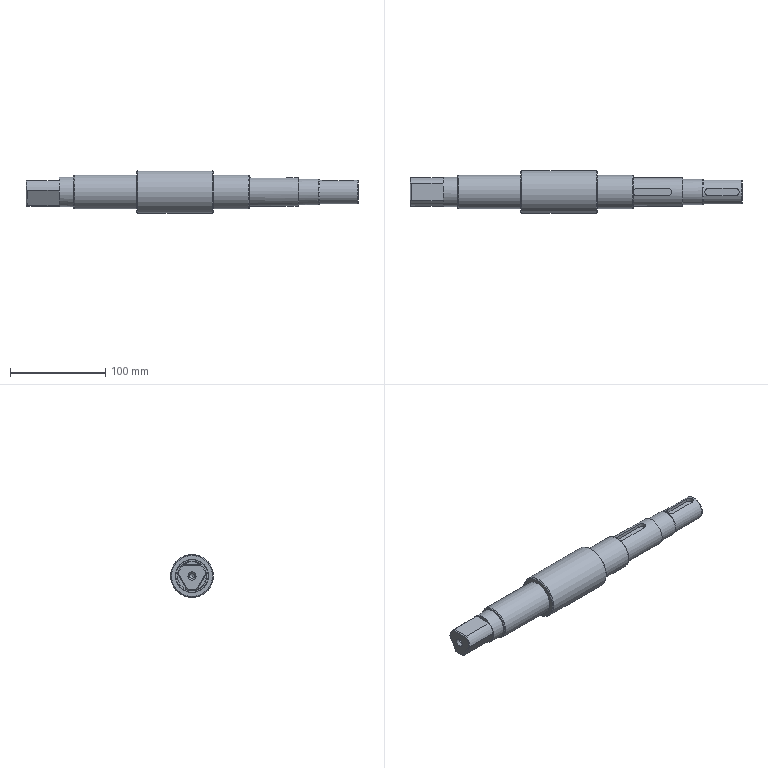NC program | NX | posted with a generic post | part box 348.4 x 45 x 45 mm
Lines 26 to 881 of 8230:
(ZLEVEL_PROFILE , TOOL : D12)
N44 T12 M6
N46 G54
N48 G17 G0 G90 X1.494 Y-21.088 B0. C0. S3000 M3
N50 G43 Z30. H12
N52 Z3.
N54 G94 G1 X0.322 Y-21.168 Z2.969 F1000.
N56 X-0.867 Y-21.132 Z2.938
N58 X-2.032 Y-21.052 Z2.908
N60 X-3.191 Y-20.908 Z2.877
N62 X-3.454 Y-20.866 Z2.87
N64 X-5.417 Y-20.445 Z2.817
N66 X-6.627 Y-20.109 Z2.785
N68 X-6.926 Y-20.009 Z2.776
N70 X-8.672 Y-19.316 Z2.727
N72 X-9.737 Y-18.63 Z2.694
N74 X-10.648 Y-17.751 Z2.661
N76 X-11.005 Y-17.24 Z2.644
N78 X-20.329 Y-1.089 Z2.156
N80 X-20.615 Y-0.558 Z2.14
N82 X-20.993 Y0.754 Z2.105
N84 X-21.068 Y2.117 Z2.069
N86 X-20.974 Y2.712 Z2.053
N88 X-20.913 Y3.155 Z2.041
N90 X-20.759 Y4.101 Z2.016
N92 X-20.487 Y5.346 Z1.983
N94 X-19.903 Y7.245 Z1.931
N96 X-19.428 Y8.428 Z1.897
N98 X-18.84 Y9.668 Z1.861
N100 X-18.585 Y10.139 Z1.847
N102 X-17.871 Y11.312 Z1.811
N104 X-17.235 Y12.297 Z1.781
N106 X-16.077 Y13.775 Z1.732
N108 X-14.802 Y15.153 Z1.682
N110 X-13.929 Y15.937 Z1.652
N112 X-12.824 Y16.819 Z1.615
N114 X-12.649 Y16.951 Z1.609
N116 X-12.159 Y17.312 Z1.593
N118 X-10.915 Y17.876 Z1.557
N120 X-9.578 Y18.153 Z1.522
N122 X-8.97 Y18.15 Z1.506
N124 X9.215 Z1.029
N126 X9.824 Y18.127 Z1.013
N128 X11.056 Y17.828 Z0.98
N130 X12.202 Y17.286 Z0.947
N132 X12.69 Y16.92 Z0.931
N134 X13.605 Y16.224 Z0.901
N136 X15.197 Y14.736 Z0.844
N138 X16.634 Y13.098 Z0.787
N140 X17.902 Y11.327 Z0.73
N142 X18.473 Y10.329 Z0.7
N144 X19.156 Y9.011 Z0.661
N146 X19.696 Y7.705 Z0.624
N148 X19.848 Y7.306 Z0.613
N150 X20.415 Y5.527 Z0.564
N152 X20.715 Y4.405 Z0.533
N154 X20.838 Y3.786 Z0.517
N156 X21.068 Y2.023 Z0.47
N158 X20.986 Y0.776 Z0.438
N160 X20.663 Y-0.43 Z0.405
N162 X20.39 Y-0.984 Z0.389
N164 X11.114 Y-17.05 Z-0.097
N166 X10.802 Y-17.561 Z-0.113
N168 X9.86 Y-18.549 Z-0.149
N170 X8.718 Y-19.298 Z-0.184
N172 X8.159 Y-19.512 Z-0.2
N174 X7.072 Y-19.96 F2200.
N176 G2 X3.724 Y-20.82 R30.718
N178 X-0.867 Y-21.132 R23.572
N180 X-3.191 Y-20.908 R42.566
N182 G1 X-3.454 Y-20.866
N184 X-5.417 Y-20.445
N186 G2 X-8.093 Y-19.546 R26.263
N188 X-11.005 Y-17.24 R6.45
N190 G1 X-20.329 Y-1.089
N192 G2 X-20.974 Y2.712 R6.027
N194 G1 X-20.913 Y3.155
N196 X-20.759 Y4.101
N198 G2 X-19.428 Y8.428 R27.054
N200 X-17.871 Y11.312 R31.394
N202 X-13.929 Y15.937 R22.915
N204 G1 X-12.824 Y16.819
N206 X-12.649 Y16.951
N208 G2 X-8.97 Y18.15 R6.146
N210 G1 X9.215
N212 G2 X12.69 Y16.92 R6.187
N214 X18.473 Y10.329 R22.033
N216 X19.696 Y7.705 R33.258
N218 G1 X19.848 Y7.306
N220 X20.415 Y5.527
N222 G2 X20.988 Y2.635 R22.446
N224 X20.39 Y-0.984 R6.331
N226 G1 X11.114 Y-17.05
N228 G2 X8.159 Y-19.512 R5.953
N230 G1 X7.78 Y-19.667 Z-0.207
N232 X7.395 Y-19.808 Z-0.214
N234 X7.009 Y-19.939 Z-0.221
N236 X6.625 Y-20.074 Z-0.229
N238 X6.238 Y-20.209 Z-0.236
N240 X5.846 Y-20.326 Z-0.243
N242 X5.451 Y-20.434 Z-0.25
N244 X5.051 Y-20.52 Z-0.257
N246 X4.651 Y-20.609 Z-0.264
N248 X4.252 Y-20.698 Z-0.271
N250 X3.853 Y-20.789 Z-0.279
N252 X3.451 Y-20.867 Z-0.286
N254 X3.046 Y-20.922 Z-0.293
N256 X2.639 Y-20.965 Z-0.3
N258 X2.232 Y-21.01 Z-0.307
N260 X1.826 Y-21.055 Z-0.314
N262 X1.418 Y-21.1 Z-0.321
N264 X1.01 Y-21.125 Z-0.329
N266 X0.601 Y-21.13 Z-0.336
N268 X0.191 Y-21.128 Z-0.343
N270 X-0.218 Z-0.35
N272 X-0.627 Y-21.13 Z-0.357
N274 X-1.036 Y-21.124 Z-0.364
N276 X-1.444 Y-21.098 Z-0.371
N278 X-1.851 Y-21.052 Z-0.379
N280 X-2.258 Y-21.007 Z-0.386
N282 X-2.665 Y-20.962 Z-0.393
N284 X-3.072 Y-20.923 Z-0.4
N286 X-3.191 Y-20.908
N288 X-3.454 Y-20.866
N290 X-5.417 Y-20.445
N292 G2 X-8.095 Y-19.545 R26.183
N294 X-11.004 Y-17.24 R6.449
N296 G1 X-20.329 Y-1.089
N298 G2 X-20.974 Y2.712 R6.027
N300 G1 X-20.913 Y3.155
N302 X-20.759 Y4.101
N304 G2 X-19.428 Y8.429 R27.032
N306 X-17.871 Y11.312 R31.353
N308 X-13.926 Y15.939 R22.888
N310 G1 X-12.824 Y16.819
N312 X-12.649 Y16.951
N314 G2 X-8.97 Y18.15 R6.146
N316 G1 X9.215
N318 G2 X12.69 Y16.92 R6.187
N320 X18.475 Y10.326 R22.025
N322 X19.696 Y7.705 R33.111
N324 G1 X19.848 Y7.306
N326 X20.415 Y5.527
N328 G2 X20.988 Y2.634 R22.427
N330 X20.39 Y-0.983 R6.332
N332 G1 X11.114 Y-17.05
N334 G2 X8.159 Y-19.512 R5.953
N336 G1 X7.78 Y-19.667 Z-0.407
N338 X7.395 Y-19.808 Z-0.414
N340 X7.009 Y-19.939 Z-0.421
N342 X6.625 Y-20.074 Z-0.429
N344 X6.238 Y-20.209 Z-0.436
N346 X5.846 Y-20.326 Z-0.443
N348 X5.451 Y-20.434 Z-0.45
N350 X5.051 Y-20.52 Z-0.457
N352 X4.651 Y-20.609 Z-0.464
N354 X4.252 Y-20.698 Z-0.471
N356 X3.853 Y-20.79 Z-0.479
N358 X3.451 Y-20.867 Z-0.486
N360 X3.046 Y-20.922 Z-0.493
N362 X2.639 Y-20.965 Z-0.5
N364 X2.232 Y-21.01 Z-0.507
N366 X1.826 Y-21.055 Z-0.514
N368 X1.419 Y-21.101 Z-0.521
N370 X1.01 Y-21.125 Z-0.529
N372 X0.601 Y-21.13 Z-0.536
N374 X0.191 Y-21.128 Z-0.543
N376 X-0.218 Z-0.55
N378 X-0.627 Y-21.13 Z-0.557
N380 X-1.036 Y-21.124 Z-0.564
N382 X-1.444 Y-21.098 Z-0.571
N384 X-1.851 Y-21.052 Z-0.579
N386 X-2.258 Y-21.007 Z-0.586
N388 X-2.665 Y-20.962 Z-0.593
N390 X-3.072 Y-20.923 Z-0.6
N392 X-3.191 Y-20.908
N394 X-3.454 Y-20.866
N396 X-5.417 Y-20.445
N398 G2 X-8.097 Y-19.544 R26.105
N400 X-11.004 Y-17.24 R6.448
N402 G1 X-20.329 Y-1.089
N404 G2 X-20.974 Y2.712 R6.027
N406 G1 X-20.913 Y3.155
N408 X-20.759 Y4.101
N410 G2 X-19.427 Y8.43 R27.01
N412 X-17.871 Y11.312 R31.313
N414 X-13.923 Y15.942 R22.861
N416 G1 X-12.824 Y16.819
N418 X-12.649 Y16.951
N420 G2 X-8.97 Y18.15 R6.146
N422 G1 X9.215
N424 G2 X12.69 Y16.92 R6.186
N426 X18.476 Y10.324 R22.016
N428 X19.696 Y7.705 R32.965
N430 G1 X19.848 Y7.306
N432 X20.415 Y5.527
N434 G2 X20.988 Y2.633 R22.408
N436 X20.39 Y-0.983 R6.332
N438 G1 X11.114 Y-17.05
N440 G2 X8.159 Y-19.512 R5.953
N442 G1 X7.78 Y-19.667 Z-0.607
N444 X7.396 Y-19.808 Z-0.614
N446 X7.009 Y-19.939 Z-0.621
N448 X6.625 Y-20.075 Z-0.629
N450 X6.237 Y-20.208 Z-0.636
N452 X5.846 Y-20.326 Z-0.643
N454 X5.451 Y-20.434 Z-0.65
N456 X5.051 Y-20.521 Z-0.657
N458 X4.651 Y-20.61 Z-0.664
N460 X4.252 Y-20.698 Z-0.671
N462 X3.853 Y-20.789 Z-0.679
N464 X3.451 Y-20.867 Z-0.686
N466 X3.046 Y-20.923 Z-0.693
N468 X2.639 Y-20.965 Z-0.7
N470 X2.232 Y-21.01 Z-0.707
N472 X1.826 Y-21.054 Z-0.714
N474 X1.419 Y-21.101 Z-0.721
N476 X1.01 Y-21.125 Z-0.729
N478 X0.601 Y-21.13 Z-0.736
N480 X0.191 Y-21.128 Z-0.743
N482 X-0.218 Z-0.75
N484 X-0.627 Y-21.13 Z-0.757
N486 X-1.036 Y-21.124 Z-0.764
N488 X-1.444 Y-21.098 Z-0.771
N490 X-1.851 Y-21.052 Z-0.779
N492 X-2.258 Y-21.007 Z-0.786
N494 X-2.665 Y-20.962 Z-0.793
N496 X-3.072 Y-20.923 Z-0.8
N498 X-3.191 Y-20.908
N500 X-3.454 Y-20.866
N502 X-5.417 Y-20.445
N504 G2 X-8.099 Y-19.543 R26.026
N506 X-11.004 Y-17.24 R6.447
N508 G1 X-20.329 Y-1.089
N510 G2 X-20.974 Y2.712 R6.027
N512 G1 X-20.913 Y3.155
N514 X-20.759 Y4.101
N516 G2 X-19.427 Y8.431 R26.988
N518 X-17.871 Y11.312 R31.273
N520 X-13.919 Y15.945 R22.834
N522 G1 X-12.824 Y16.819
N524 X-12.649 Y16.951
N526 G2 X-8.97 Y18.15 R6.146
N528 G1 X9.215
N530 G2 X12.69 Y16.92 R6.186
N532 X18.477 Y10.321 R22.007
N534 X19.696 Y7.705 R32.82
N536 G1 X19.848 Y7.306
N538 X20.415 Y5.527
N540 G2 X20.988 Y2.633 R22.389
N542 X20.391 Y-0.982 R6.332
N544 G1 X11.114 Y-17.05
N546 G2 X8.159 Y-19.512 R5.953
N548 G1 X7.78 Y-19.667 Z-0.807
N550 X7.395 Y-19.808 Z-0.814
N552 X7.009 Y-19.94 Z-0.821
N554 X6.625 Y-20.074 Z-0.829
N556 X6.237 Y-20.208 Z-0.836
N558 X5.846 Y-20.326 Z-0.843
N560 X5.451 Y-20.433 Z-0.85
N562 X5.051 Y-20.521 Z-0.857
N564 X4.651 Y-20.61 Z-0.864
N566 X4.252 Y-20.698 Z-0.871
N568 X3.853 Y-20.789 Z-0.879
N570 X3.451 Y-20.867 Z-0.886
N572 X3.046 Y-20.923 Z-0.893
N574 X2.639 Y-20.965 Z-0.9
N576 X2.232 Y-21.009 Z-0.907
N578 X1.826 Y-21.055 Z-0.914
N580 X1.419 Y-21.101 Z-0.921
N582 X1.01 Y-21.125 Z-0.929
N584 X0.601 Y-21.13 Z-0.936
N586 X0.192 Y-21.138 Z-0.943
N588 X-0.218 Y-21.14 Z-0.95
N590 X-0.627 Y-21.134 Z-0.957
N592 X-1.036 Y-21.124 Z-0.964
N594 X-1.444 Y-21.099 Z-0.971
N596 X-1.853 Y-21.067 Z-0.979
N598 X-2.26 Y-21.027 Z-0.986
N600 X-2.666 Y-20.98 Z-0.993
N602 X-3.072 Y-20.926 Z-1.
N604 G2 X-8.273 Y-19.465 R21.135
N606 X-11.134 Y-17.015 R6.16
N608 G1 X-20.329 Y-1.089
N610 G2 X-20.974 Y2.712 R6.027
N612 G1 X-20.909 Y3.178
N614 X-20.881 Y3.365
N616 G2 X-12.649 Y16.951 R21.153
N618 X-8.97 Y18.15 R6.146
N620 G1 X9.215
N622 G2 X12.69 Y16.92 R6.186
N624 X20.995 Y2.56 R21.15
N626 X20.839 Y0.226 R6.123
N628 X20.203 Y-1.307 R6.281
N630 G1 X11.114 Y-17.05
N632 G2 X8.159 Y-19.512 R5.953
N634 G1 X7.78 Y-19.667 Z-1.007
N636 X7.398 Y-19.814 Z-1.014
N638 X7.013 Y-19.953 Z-1.021
N640 X6.626 Y-20.085 Z-1.029
N642 X6.236 Y-20.21 Z-1.036
N644 X5.844 Y-20.327 Z-1.043
N646 X5.449 Y-20.436 Z-1.05
N648 X5.053 Y-20.538 Z-1.057
N650 X4.655 Y-20.631 Z-1.064
N652 X4.255 Y-20.718 Z-1.071
N654 X3.853 Y-20.796 Z-1.079
N656 X3.45 Y-20.867 Z-1.086
N658 X3.046 Y-20.93 Z-1.093
N660 X2.64 Y-20.985 Z-1.1
N662 X2.234 Y-21.032 Z-1.107
N664 X1.826 Y-21.071 Z-1.114
N666 X1.418 Y-21.102 Z-1.121
N668 X1.01 Y-21.126 Z-1.129
N670 X0.601 Y-21.141 Z-1.136
N672 X0.192 Y-21.149 Z-1.143
N674 X-0.218 Z-1.15
N676 X-0.627 Y-21.141 Z-1.157
N678 X-1.036 Y-21.125 Z-1.164
N680 X-1.444 Y-21.101 Z-1.171
N682 X-1.852 Y-21.069 Z-1.179
N684 X-2.259 Y-21.029 Z-1.186
N686 X-2.666 Y-20.981 Z-1.193
N688 X-3.071 Y-20.926 Z-1.2
N690 G2 X-8.273 Y-19.465 R21.15
N692 X-11.135 Y-17.013 R6.159
N694 G1 X-20.329 Y-1.089
N696 G2 X-20.974 Y2.712 R6.027
N698 G1 X-20.958 Y2.84
N700 G2 X-12.824 Y16.819 R21.15
N702 X-9.005 Y18.15 R6.32
N704 G1 X9.215
N706 G2 X12.671 Y16.934 R6.186
N708 X20.995 Y2.56 R21.15
N710 X20.839 Y0.226 R5.624
N712 X20.203 Y-1.307 R6.717
N714 G1 X11.114 Y-17.05
N716 G2 X8.159 Y-19.512 R5.953
N718 G1 X7.78 Y-19.667 Z-1.207
N720 X7.398 Y-19.814 Z-1.214
N722 X7.013 Y-19.953 Z-1.221
N724 X6.626 Y-20.085 Z-1.229
N726 X6.236 Y-20.21 Z-1.236
N728 X5.844 Y-20.327 Z-1.243
N730 X5.45 Y-20.436 Z-1.25
N732 X5.053 Y-20.537 Z-1.257
N734 X4.655 Y-20.631 Z-1.264
N736 X4.255 Y-20.718 Z-1.271
N738 X3.853 Y-20.796 Z-1.279
N740 X3.45 Y-20.867 Z-1.286
N742 X3.046 Y-20.93 Z-1.293
N744 X2.64 Y-20.985 Z-1.3
N746 X2.234 Y-21.032 Z-1.307
N748 X1.827 Y-21.071 Z-1.314
N750 X1.419 Y-21.102 Z-1.321
N752 X1.01 Y-21.126 Z-1.329
N754 X0.601 Y-21.141 Z-1.336
N756 X0.192 Y-21.149 Z-1.343
N758 X-0.217 Z-1.35
N760 X-0.626 Y-21.141 Z-1.357
N762 X-1.035 Y-21.125 Z-1.364
N764 X-1.444 Y-21.101 Z-1.371
N766 X-1.852 Y-21.069 Z-1.379
N768 X-2.259 Y-21.029 Z-1.386
N770 X-2.665 Y-20.981 Z-1.393
N772 X-3.071 Y-20.926 Z-1.4
N774 G2 X-8.273 Y-19.465 R21.15
N776 X-11.136 Y-17.012 R6.159
N778 G1 X-20.329 Y-1.089
N780 G2 X-20.985 Y2.636 R5.935
N782 X-12.776 Y16.855 R21.15
N784 X-9.005 Y18.15 R6.257
N786 G1 X9.215
N788 G2 X12.673 Y16.933 R6.185
N790 X20.995 Y2.56 R21.15
N792 X20.839 Y0.226 R5.624
N794 X20.203 Y-1.307 R6.717
N796 G1 X11.114 Y-17.05
N798 G2 X8.159 Y-19.513 R5.955
N800 G1 X7.78 Y-19.667 Z-1.407
N802 X7.398 Y-19.814 Z-1.414
N804 X7.013 Y-19.953 Z-1.421
N806 X6.626 Y-20.085 Z-1.429
N808 X6.236 Y-20.21 Z-1.436
N810 X5.844 Y-20.327 Z-1.443
N812 X5.45 Y-20.436 Z-1.45
N814 X5.053 Y-20.537 Z-1.457
N816 X4.655 Y-20.631 Z-1.464
N818 X4.255 Y-20.718 Z-1.471
N820 X3.853 Y-20.796 Z-1.479
N822 X3.45 Y-20.867 Z-1.486
N824 X3.046 Y-20.93 Z-1.493
N826 X2.64 Y-20.985 Z-1.5
N828 X2.234 Y-21.032 Z-1.507
N830 X1.827 Y-21.071 Z-1.514
N832 X1.419 Y-21.102 Z-1.521
N834 X1.01 Y-21.126 Z-1.529
N836 X0.601 Y-21.141 Z-1.536
N838 X0.192 Y-21.149 Z-1.543
N840 X-0.217 Z-1.55
N842 X-0.626 Y-21.141 Z-1.557
N844 X-1.035 Y-21.125 Z-1.564
N846 X-1.444 Y-21.101 Z-1.571
N848 X-1.852 Y-21.069 Z-1.579
N850 X-2.259 Y-21.029 Z-1.586
N852 X-2.665 Y-20.981 Z-1.593
N854 X-3.071 Y-20.926 Z-1.6
N856 G2 X-8.308 Y-19.45 R21.15
N858 X-11.218 Y-16.869 R6.15
N860 G1 X-20.22 Y-1.279
N862 G2 X-20.998 Y2.53 R6.15
N864 X-12.69 Y16.92 R21.15
N866 X-8.97 Y18.15 R6.15
N868 G1 X9.
N870 G2 X12.69 Y16.92 R6.15
N872 X20.998 Y2.53 R21.15
N874 X20.218 Y-1.281 R6.15
N876 G1 X11.218 Y-16.87
N878 G2 X8.308 Y-19.45 R6.15
N880 G1 X8.159 Y-19.513
N882 X7.78 Y-19.667 Z-1.607
N884 X7.398 Y-19.814 Z-1.614
N886 X7.013 Y-19.953 Z-1.621
N888 X6.626 Y-20.085 Z-1.629
N890 X6.236 Y-20.21 Z-1.636
N892 X5.844 Y-20.327 Z-1.643
N894 X5.45 Y-20.436 Z-1.65
N896 X5.053 Y-20.537 Z-1.657
N898 X4.655 Y-20.631 Z-1.664
N900 X4.255 Y-20.718 Z-1.671
N902 X3.853 Y-20.796 Z-1.679
N904 X3.45 Y-20.867 Z-1.686
N906 X3.046 Y-20.93 Z-1.693
N908 X2.64 Y-20.985 Z-1.7
N910 X2.234 Y-21.032 Z-1.707
N912 X1.827 Y-21.071 Z-1.714
N914 X1.419 Y-21.102 Z-1.721
N916 X1.01 Y-21.126 Z-1.729
N918 X0.601 Y-21.141 Z-1.736
N920 X0.192 Y-21.149 Z-1.743
N922 X-0.217 Z-1.75
N924 X-0.626 Y-21.141 Z-1.757
N926 X-1.035 Y-21.125 Z-1.764
N928 X-1.444 Y-21.101 Z-1.771
N930 X-1.852 Y-21.069 Z-1.779
N932 X-2.259 Y-21.029 Z-1.786
N934 X-2.665 Y-20.981 Z-1.793
N936 X-3.071 Y-20.926 Z-1.8
N938 G2 X-8.308 Y-19.45 R21.15
N940 X-11.218 Y-16.869 R6.15
N942 G1 X-20.22 Y-1.279
N944 G2 X-20.998 Y2.53 R6.15
N946 X-12.69 Y16.92 R21.15
N948 X-8.97 Y18.15 R6.15
N950 G1 X9.
N952 G2 X12.69 Y16.92 R6.15
N954 X20.998 Y2.53 R21.15
N956 X20.218 Y-1.281 R6.15
N958 G1 X11.218 Y-16.87
N960 G2 X8.308 Y-19.45 R6.15
N962 G1 X8.159 Y-19.513
N964 X7.78 Y-19.668 Z-1.807
N966 X7.398 Y-19.814 Z-1.814
N968 X7.013 Y-19.953 Z-1.821
N970 X6.626 Y-20.085 Z-1.829
N972 X6.236 Y-20.21 Z-1.836
N974 X5.844 Y-20.327 Z-1.843
N976 X5.45 Y-20.436 Z-1.85
N978 X5.053 Y-20.537 Z-1.857
N980 X4.655 Y-20.631 Z-1.864
N982 X4.255 Y-20.718 Z-1.871
N984 X3.853 Y-20.796 Z-1.879
N986 X3.45 Y-20.867 Z-1.886
N988 X3.046 Y-20.93 Z-1.893
N990 X2.64 Y-20.985 Z-1.9
N992 X2.234 Y-21.032 Z-1.907
N994 X1.827 Y-21.071 Z-1.914
N996 X1.419 Y-21.102 Z-1.921
N998 X1.01 Y-21.126 Z-1.929
N1000 X0.601 Y-21.141 Z-1.936
N1002 X0.192 Y-21.149 Z-1.943
N1004 X-0.217 Z-1.95
N1006 X-0.626 Y-21.141 Z-1.957
N1008 X-1.035 Y-21.125 Z-1.964
N1010 X-1.444 Y-21.101 Z-1.971
N1012 X-1.852 Y-21.069 Z-1.979
N1014 X-2.259 Y-21.029 Z-1.986
N1016 X-2.665 Y-20.981 Z-1.993
N1018 X-3.071 Y-20.926 Z-2.
N1020 G2 X-8.308 Y-19.45 R21.15
N1022 X-11.218 Y-16.869 R6.15
N1024 G1 X-20.22 Y-1.278
N1026 G2 X-20.998 Y2.53 R6.15
N1028 X-12.69 Y16.92 R21.15
N1030 X-8.97 Y18.15 R6.15
N1032 G1 X9.
N1034 G2 X12.69 Y16.92 R6.15
N1036 X20.998 Y2.53 R21.15
N1038 X20.218 Y-1.281 R6.15
N1040 G1 X11.218 Y-16.87
N1042 G2 X8.308 Y-19.45 R6.15
N1044 G1 X8.159 Y-19.513
N1046 X7.78 Y-19.668 Z-2.007
N1048 X7.398 Y-19.814 Z-2.014
N1050 X7.013 Y-19.953 Z-2.021
N1052 X6.626 Y-20.085 Z-2.029
N1054 X6.236 Y-20.21 Z-2.036
N1056 X5.844 Y-20.327 Z-2.043
N1058 X5.45 Y-20.436 Z-2.05
N1060 X5.053 Y-20.537 Z-2.057
N1062 X4.655 Y-20.631 Z-2.064
N1064 X4.255 Y-20.718 Z-2.071
N1066 X3.853 Y-20.796 Z-2.079
N1068 X3.45 Y-20.867 Z-2.086
N1070 X3.046 Y-20.93 Z-2.093
N1072 X2.64 Y-20.985 Z-2.1
N1074 X2.234 Y-21.032 Z-2.107
N1076 X1.827 Y-21.071 Z-2.114
N1078 X1.419 Y-21.102 Z-2.121
N1080 X1.01 Y-21.126 Z-2.129
N1082 X0.601 Y-21.141 Z-2.136
N1084 X0.192 Y-21.149 Z-2.143
N1086 X-0.217 Z-2.15
N1088 X-0.626 Y-21.141 Z-2.157
N1090 X-1.035 Y-21.125 Z-2.164
N1092 X-1.444 Y-21.101 Z-2.171
N1094 X-1.852 Y-21.069 Z-2.179
N1096 X-2.259 Y-21.029 Z-2.186
N1098 X-2.665 Y-20.981 Z-2.193
N1100 X-3.071 Y-20.926 Z-2.2
N1102 G2 X-8.308 Y-19.45 R21.15
N1104 X-11.218 Y-16.869 R6.15
N1106 G1 X-20.22 Y-1.278
N1108 G2 X-20.998 Y2.53 R6.15
N1110 X-12.69 Y16.92 R21.15
N1112 X-8.97 Y18.15 R6.15
N1114 G1 X9.
N1116 G2 X12.69 Y16.92 R6.15
N1118 X20.998 Y2.53 R21.15
N1120 X20.218 Y-1.281 R6.15
N1122 G1 X11.218 Y-16.87
N1124 G2 X8.308 Y-19.45 R6.15
N1126 G1 X8.159 Y-19.513
N1128 X7.78 Y-19.668 Z-2.207
N1130 X7.398 Y-19.814 Z-2.214
N1132 X7.013 Y-19.953 Z-2.221
N1134 X6.626 Y-20.085 Z-2.229
N1136 X6.236 Y-20.21 Z-2.236
N1138 X5.844 Y-20.327 Z-2.243
N1140 X5.45 Y-20.436 Z-2.25
N1142 X5.053 Y-20.537 Z-2.257
N1144 X4.655 Y-20.631 Z-2.264
N1146 X4.255 Y-20.718 Z-2.271
N1148 X3.853 Y-20.796 Z-2.279
N1150 X3.45 Y-20.867 Z-2.286
N1152 X3.046 Y-20.93 Z-2.293
N1154 X2.64 Y-20.985 Z-2.3
N1156 X2.234 Y-21.032 Z-2.307
N1158 X1.827 Y-21.071 Z-2.314
N1160 X1.419 Y-21.102 Z-2.321
N1162 X1.01 Y-21.126 Z-2.329
N1164 X0.601 Y-21.141 Z-2.336
N1166 X0.192 Y-21.149 Z-2.343
N1168 X-0.217 Z-2.35
N1170 X-0.626 Y-21.141 Z-2.357
N1172 X-1.035 Y-21.125 Z-2.364
N1174 X-1.444 Y-21.101 Z-2.371
N1176 X-1.852 Y-21.069 Z-2.379
N1178 X-2.259 Y-21.029 Z-2.386
N1180 X-2.665 Y-20.981 Z-2.393
N1182 X-3.071 Y-20.926 Z-2.4
N1184 G2 X-8.308 Y-19.45 R21.15
N1186 X-11.218 Y-16.869 R6.15
N1188 G1 X-20.22 Y-1.278
N1190 G2 X-20.998 Y2.53 R6.15
N1192 X-12.69 Y16.92 R21.15
N1194 X-8.97 Y18.15 R6.15
N1196 G1 X9.
N1198 G2 X12.69 Y16.92 R6.15
N1200 X20.998 Y2.53 R21.15
N1202 X20.218 Y-1.281 R6.15
N1204 G1 X11.218 Y-16.87
N1206 G2 X8.308 Y-19.45 R6.15
N1208 G1 X8.159 Y-19.513
N1210 X7.78 Y-19.668 Z-2.407
N1212 X7.398 Y-19.814 Z-2.414
N1214 X7.013 Y-19.953 Z-2.421
N1216 X6.626 Y-20.085 Z-2.429
N1218 X6.236 Y-20.21 Z-2.436
N1220 X5.844 Y-20.327 Z-2.443
N1222 X5.45 Y-20.436 Z-2.45
N1224 X5.053 Y-20.537 Z-2.457
N1226 X4.655 Y-20.631 Z-2.464
N1228 X4.255 Y-20.718 Z-2.471
N1230 X3.853 Y-20.796 Z-2.479
N1232 X3.45 Y-20.867 Z-2.486
N1234 X3.046 Y-20.93 Z-2.493
N1236 X2.64 Y-20.985 Z-2.5
N1238 X2.234 Y-21.032 Z-2.507
N1240 X1.827 Y-21.071 Z-2.514
N1242 X1.419 Y-21.102 Z-2.521
N1244 X1.01 Y-21.126 Z-2.529
N1246 X0.601 Y-21.141 Z-2.536
N1248 X0.192 Y-21.149 Z-2.543
N1250 X-0.217 Z-2.55
N1252 X-0.626 Y-21.141 Z-2.557
N1254 X-1.035 Y-21.125 Z-2.564
N1256 X-1.444 Y-21.101 Z-2.571
N1258 X-1.852 Y-21.069 Z-2.579
N1260 X-2.259 Y-21.029 Z-2.586
N1262 X-2.665 Y-20.981 Z-2.593
N1264 X-3.071 Y-20.926 Z-2.6
N1266 G2 X-8.308 Y-19.45 R21.15
N1268 X-11.218 Y-16.869 R6.15
N1270 G1 X-20.22 Y-1.278
N1272 G2 X-20.998 Y2.53 R6.15
N1274 X-12.69 Y16.92 R21.15
N1276 X-8.97 Y18.15 R6.15
N1278 G1 X9.
N1280 G2 X12.69 Y16.92 R6.15
N1282 X20.998 Y2.53 R21.15
N1284 X20.218 Y-1.281 R6.15
N1286 G1 X11.218 Y-16.871
N1288 G2 X8.308 Y-19.45 R6.15
N1290 G1 X8.159 Y-19.513
N1292 X7.78 Y-19.668 Z-2.607
N1294 X7.398 Y-19.814 Z-2.614
N1296 X7.013 Y-19.953 Z-2.621
N1298 X6.626 Y-20.085 Z-2.629
N1300 X6.236 Y-20.21 Z-2.636
N1302 X5.844 Y-20.327 Z-2.643
N1304 X5.45 Y-20.436 Z-2.65
N1306 X5.053 Y-20.537 Z-2.657
N1308 X4.655 Y-20.631 Z-2.664
N1310 X4.255 Y-20.718 Z-2.671
N1312 X3.853 Y-20.796 Z-2.679
N1314 X3.45 Y-20.867 Z-2.686
N1316 X3.046 Y-20.93 Z-2.693
N1318 X2.64 Y-20.985 Z-2.7
N1320 X2.234 Y-21.032 Z-2.707
N1322 X1.827 Y-21.071 Z-2.714
N1324 X1.419 Y-21.102 Z-2.721
N1326 X1.01 Y-21.126 Z-2.729
N1328 X0.601 Y-21.141 Z-2.736
N1330 X0.192 Y-21.149 Z-2.743
N1332 X-0.217 Z-2.75
N1334 X-0.626 Y-21.141 Z-2.757
N1336 X-1.035 Y-21.125 Z-2.764
N1338 X-1.444 Y-21.101 Z-2.771
N1340 X-1.852 Y-21.069 Z-2.779
N1342 X-2.259 Y-21.029 Z-2.786
N1344 X-2.665 Y-20.981 Z-2.793
N1346 X-3.071 Y-20.926 Z-2.8
N1348 G2 X-8.308 Y-19.45 R21.15
N1350 X-11.218 Y-16.869 R6.15
N1352 G1 X-20.22 Y-1.278
N1354 G2 X-20.998 Y2.53 R6.15
N1356 X-12.69 Y16.92 R21.15
N1358 X-8.97 Y18.15 R6.15
N1360 G1 X9.
N1362 G2 X12.69 Y16.92 R6.15
N1364 X20.998 Y2.53 R21.15
N1366 X20.218 Y-1.281 R6.15
N1368 G1 X11.218 Y-16.871
N1370 G2 X8.308 Y-19.45 R6.15
N1372 G1 X8.159 Y-19.513
N1374 X7.78 Y-19.668 Z-2.807
N1376 X7.398 Y-19.814 Z-2.814
N1378 X7.013 Y-19.953 Z-2.821
N1380 X6.626 Y-20.085 Z-2.829
N1382 X6.236 Y-20.21 Z-2.836
N1384 X5.844 Y-20.327 Z-2.843
N1386 X5.45 Y-20.436 Z-2.85
N1388 X5.053 Y-20.537 Z-2.857
N1390 X4.655 Y-20.631 Z-2.864
N1392 X4.255 Y-20.718 Z-2.871
N1394 X3.853 Y-20.796 Z-2.879
N1396 X3.45 Y-20.867 Z-2.886
N1398 X3.046 Y-20.93 Z-2.893
N1400 X2.64 Y-20.985 Z-2.9
N1402 X2.234 Y-21.032 Z-2.907
N1404 X1.827 Y-21.071 Z-2.914
N1406 X1.419 Y-21.102 Z-2.921
N1408 X1.01 Y-21.126 Z-2.929
N1410 X0.601 Y-21.141 Z-2.936
N1412 X0.192 Y-21.149 Z-2.943
N1414 X-0.217 Z-2.95
N1416 X-0.626 Y-21.141 Z-2.957
N1418 X-1.035 Y-21.125 Z-2.964
N1420 X-1.444 Y-21.101 Z-2.971
N1422 X-1.852 Y-21.069 Z-2.979
N1424 X-2.259 Y-21.029 Z-2.986
N1426 X-2.665 Y-20.981 Z-2.993
N1428 X-3.071 Y-20.926 Z-3.
N1430 G2 X-8.308 Y-19.45 R21.15
N1432 X-11.218 Y-16.869 R6.15
N1434 G1 X-20.22 Y-1.278
N1436 G2 X-20.998 Y2.53 R6.15
N1438 X-12.69 Y16.92 R21.15
N1440 X-8.97 Y18.15 R6.15
N1442 G1 X9.
N1444 G2 X12.69 Y16.92 R6.15
N1446 X20.998 Y2.53 R21.15
N1448 X20.218 Y-1.281 R6.15
N1450 G1 X11.217 Y-16.871
N1452 G2 X8.308 Y-19.45 R6.15
N1454 G1 X8.159 Y-19.513
N1456 X7.78 Y-19.668 Z-3.007
N1458 X7.398 Y-19.814 Z-3.014
N1460 X7.013 Y-19.953 Z-3.021
N1462 X6.626 Y-20.085 Z-3.029
N1464 X6.236 Y-20.21 Z-3.036
N1466 X5.844 Y-20.327 Z-3.043
N1468 X5.45 Y-20.436 Z-3.05
N1470 X5.053 Y-20.537 Z-3.057
N1472 X4.655 Y-20.631 Z-3.064
N1474 X4.255 Y-20.718 Z-3.071
N1476 X3.853 Y-20.796 Z-3.079
N1478 X3.45 Y-20.867 Z-3.086
N1480 X3.046 Y-20.93 Z-3.093
N1482 X2.64 Y-20.985 Z-3.1
N1484 X2.234 Y-21.032 Z-3.107
N1486 X1.827 Y-21.071 Z-3.114
N1488 X1.419 Y-21.102 Z-3.121
N1490 X1.01 Y-21.126 Z-3.129
N1492 X0.601 Y-21.141 Z-3.136
N1494 X0.192 Y-21.149 Z-3.143
N1496 X-0.217 Z-3.15
N1498 X-0.626 Y-21.141 Z-3.157
N1500 X-1.035 Y-21.125 Z-3.164
N1502 X-1.444 Y-21.101 Z-3.171
N1504 X-1.852 Y-21.069 Z-3.179
N1506 X-2.259 Y-21.029 Z-3.186
N1508 X-2.665 Y-20.981 Z-3.193
N1510 X-3.071 Y-20.926 Z-3.2
N1512 G2 X-8.308 Y-19.45 R21.15
N1514 X-11.218 Y-16.869 R6.15
N1516 G1 X-20.22 Y-1.278
N1518 G2 X-20.998 Y2.53 R6.15
N1520 X-12.69 Y16.92 R21.15
N1522 X-8.97 Y18.15 R6.15
N1524 G1 X9.
N1526 G2 X12.69 Y16.92 R6.15
N1528 X20.998 Y2.53 R21.15
N1530 X20.218 Y-1.281 R6.15
N1532 G1 X11.217 Y-16.871
N1534 G2 X8.308 Y-19.45 R6.15
N1536 G1 X8.159 Y-19.513
N1538 X7.78 Y-19.668 Z-3.207
N1540 X7.398 Y-19.814 Z-3.214
N1542 X7.013 Y-19.953 Z-3.221
N1544 X6.626 Y-20.085 Z-3.229
N1546 X6.236 Y-20.21 Z-3.236
N1548 X5.844 Y-20.327 Z-3.243
N1550 X5.45 Y-20.436 Z-3.25
N1552 X5.053 Y-20.537 Z-3.257
N1554 X4.655 Y-20.631 Z-3.264
N1556 X4.255 Y-20.718 Z-3.271
N1558 X3.853 Y-20.796 Z-3.279
N1560 X3.45 Y-20.867 Z-3.286
N1562 X3.046 Y-20.93 Z-3.293
N1564 X2.64 Y-20.985 Z-3.3
N1566 X2.234 Y-21.032 Z-3.307
N1568 X1.827 Y-21.071 Z-3.314
N1570 X1.419 Y-21.102 Z-3.321
N1572 X1.01 Y-21.126 Z-3.329
N1574 X0.601 Y-21.141 Z-3.336
N1576 X0.192 Y-21.149 Z-3.343
N1578 X-0.217 Z-3.35
N1580 X-0.626 Y-21.141 Z-3.357
N1582 X-1.035 Y-21.125 Z-3.364
N1584 X-1.444 Y-21.101 Z-3.371
N1586 X-1.852 Y-21.069 Z-3.379
N1588 X-2.259 Y-21.029 Z-3.386
N1590 X-2.665 Y-20.981 Z-3.393
N1592 X-3.071 Y-20.926 Z-3.4
N1594 G2 X-8.308 Y-19.45 R21.15
N1596 X-11.218 Y-16.869 R6.15
N1598 G1 X-20.22 Y-1.278
N1600 G2 X-20.998 Y2.53 R6.15
N1602 X-12.69 Y16.92 R21.15
N1604 X-8.97 Y18.15 R6.15
N1606 G1 X9.
N1608 G2 X12.69 Y16.92 R6.15
N1610 X20.998 Y2.53 R21.15
N1612 X20.218 Y-1.281 R6.15
N1614 G1 X11.217 Y-16.871
N1616 G2 X8.308 Y-19.45 R6.15
N1618 G1 X8.159 Y-19.513
N1620 X7.78 Y-19.668 Z-3.407
N1622 X7.398 Y-19.814 Z-3.414
N1624 X7.013 Y-19.953 Z-3.421
N1626 X6.626 Y-20.085 Z-3.429
N1628 X6.236 Y-20.21 Z-3.436
N1630 X5.844 Y-20.327 Z-3.443
N1632 X5.45 Y-20.436 Z-3.45
N1634 X5.053 Y-20.537 Z-3.457
N1636 X4.655 Y-20.631 Z-3.464
N1638 X4.255 Y-20.718 Z-3.471
N1640 X3.853 Y-20.796 Z-3.479
N1642 X3.45 Y-20.867 Z-3.486
N1644 X3.046 Y-20.93 Z-3.493
N1646 X2.64 Y-20.985 Z-3.5
N1648 X2.234 Y-21.032 Z-3.507
N1650 X1.827 Y-21.071 Z-3.514
N1652 X1.419 Y-21.102 Z-3.521
N1654 X1.01 Y-21.126 Z-3.529
N1656 X0.601 Y-21.141 Z-3.536
N1658 X0.192 Y-21.149 Z-3.543
N1660 X-0.217 Z-3.55
N1662 X-0.626 Y-21.141 Z-3.557
N1664 X-1.035 Y-21.125 Z-3.564
N1666 X-1.444 Y-21.101 Z-3.571
N1668 X-1.852 Y-21.069 Z-3.579
N1670 X-2.259 Y-21.029 Z-3.586
N1672 X-2.665 Y-20.981 Z-3.593
N1674 X-3.071 Y-20.926 Z-3.6
N1676 G2 X-8.308 Y-19.45 R21.15
N1678 X-11.218 Y-16.869 R6.15
N1680 G1 X-20.22 Y-1.278
N1682 G2 X-20.998 Y2.53 R6.15
N1684 X-12.69 Y16.92 R21.15
N1686 X-8.97 Y18.15 R6.15
N1688 G1 X9.
N1690 G2 X12.69 Y16.92 R6.15
N1692 X20.998 Y2.53 R21.15
N1694 X20.218 Y-1.281 R6.15
N1696 G1 X11.217 Y-16.871
N1698 G2 X8.308 Y-19.45 R6.15
N1700 G1 X8.159 Y-19.513
N1702 X7.78 Y-19.668 Z-3.607
N1704 X7.398 Y-19.814 Z-3.614
N1706 X7.013 Y-19.953 Z-3.621
N1708 X6.626 Y-20.085 Z-3.629
N1710 X6.236 Y-20.21 Z-3.636
N1712 X5.844 Y-20.327 Z-3.643
N1714 X5.45 Y-20.436 Z-3.65
N1716 X5.053 Y-20.537 Z-3.657
N1718 X4.655 Y-20.631 Z-3.664
N1720 X4.255 Y-20.718 Z-3.671
N1722 X3.853 Y-20.796 Z-3.679
N1724 X3.45 Y-20.867 Z-3.686
N1726 X3.046 Y-20.93 Z-3.693
N1728 X2.64 Y-20.985 Z-3.7
N1730 X2.234 Y-21.032 Z-3.707
N1732 X1.827 Y-21.071 Z-3.714
N1734 X1.419 Y-21.102 Z-3.721
N1736 X1.01 Y-21.126 Z-3.729
N1738 X0.601 Y-21.141 Z-3.736
N1740 X0.192 Y-21.149 Z-3.743
N1742 X-0.217 Z-3.75
N1744 X-0.626 Y-21.141 Z-3.757
N1746 X-1.035 Y-21.125 Z-3.764
N1748 X-1.444 Y-21.101 Z-3.771